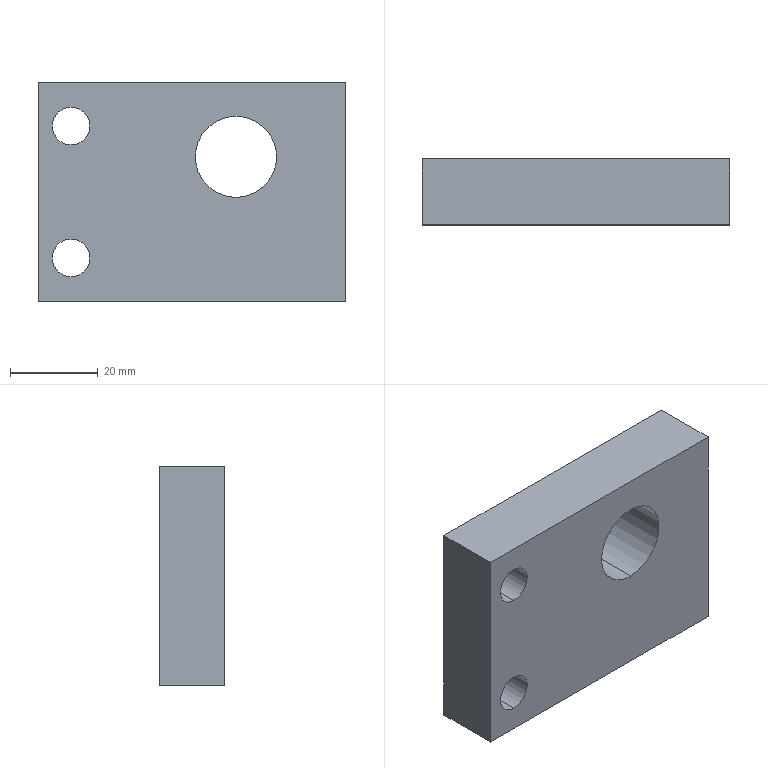Part | 1 solid | 12 faces | box 70 x 15 x 50 mm | volume 46725 mm3 | cylinder 6 | plane 6 | commonest cylinder face diameters 8.6 x4 18.5 x2
STEP:
#1=CARTESIAN_POINT('',(10.,0.,-9.75));
#2=VERTEX_POINT('',#1);
#3=CARTESIAN_POINT('',(10.,0.,8.75));
#4=VERTEX_POINT('',#3);
#5=CARTESIAN_POINT('',(10.,0.,-0.5));
#6=DIRECTION('',(0.,1.,0.));
#7=DIRECTION('',(0.,0.,1.));
#8=AXIS2_PLACEMENT_3D('',#5,#6,#7);
#9=CIRCLE('',#8,9.25);
#10=EDGE_CURVE('',#2,#4,#9,.T.);
#11=ORIENTED_EDGE('',*,*,#10,.F.);
#12=CARTESIAN_POINT('',(10.,15.,-9.75));
#13=VERTEX_POINT('',#12);
#14=CARTESIAN_POINT('',(10.,15.,-9.75));
#15=DIRECTION('',(0.,1.,0.));
#16=VECTOR('',#15,1000.);
#17=LINE('',#14,#16);
#18=EDGE_CURVE('',#2,#13,#17,.T.);
#19=ORIENTED_EDGE('',*,*,#18,.T.);
#20=CARTESIAN_POINT('',(10.,15.,8.75));
#21=VERTEX_POINT('',#20);
#22=CARTESIAN_POINT('',(10.,15.,-0.5));
#23=DIRECTION('',(0.,1.,0.));
#24=DIRECTION('',(0.,0.,1.));
#25=AXIS2_PLACEMENT_3D('',#22,#23,#24);
#26=CIRCLE('',#25,9.25);
#27=EDGE_CURVE('',#13,#21,#26,.T.);
#28=ORIENTED_EDGE('',*,*,#27,.T.);
#29=CARTESIAN_POINT('',(10.,15.,8.75));
#30=DIRECTION('',(0.,1.,0.));
#31=VECTOR('',#30,1000.);
#32=LINE('',#29,#31);
#33=EDGE_CURVE('',#4,#21,#32,.T.);
#34=ORIENTED_EDGE('',*,*,#33,.F.);
#35=EDGE_LOOP('',(#11,#19,#28,#34));
#36=FACE_OUTER_BOUND('',#35,.T.);
#37=CARTESIAN_POINT('',(10.,15.,-0.5));
#38=DIRECTION('',(0.,1.,0.));
#39=DIRECTION('',(0.,0.,1.));
#40=AXIS2_PLACEMENT_3D('',#37,#38,#39);
#41=CYLINDRICAL_SURFACE('',#40,9.25);
#42=ADVANCED_FACE('',(#36),#41,.F.);
#43=CARTESIAN_POINT('',(-27.5,0.,-27.8));
#44=VERTEX_POINT('',#43);
#45=CARTESIAN_POINT('',(-27.5,0.,-19.2));
#46=VERTEX_POINT('',#45);
#47=CARTESIAN_POINT('',(-27.5,0.,-23.5));
#48=DIRECTION('',(0.,1.,0.));
#49=DIRECTION('',(0.,0.,1.));
#50=AXIS2_PLACEMENT_3D('',#47,#48,#49);
#51=CIRCLE('',#50,4.3);
#52=EDGE_CURVE('',#44,#46,#51,.T.);
#53=ORIENTED_EDGE('',*,*,#52,.F.);
#54=CARTESIAN_POINT('',(-27.5,15.,-27.8));
#55=VERTEX_POINT('',#54);
#56=CARTESIAN_POINT('',(-27.5,0.,-27.8));
#57=DIRECTION('',(0.,1.,0.));
#58=VECTOR('',#57,1000.);
#59=LINE('',#56,#58);
#60=EDGE_CURVE('',#44,#55,#59,.T.);
#61=ORIENTED_EDGE('',*,*,#60,.T.);
#62=CARTESIAN_POINT('',(-27.5,15.,-19.2));
#63=VERTEX_POINT('',#62);
#64=CARTESIAN_POINT('',(-27.5,15.,-23.5));
#65=DIRECTION('',(0.,1.,0.));
#66=DIRECTION('',(0.,0.,1.));
#67=AXIS2_PLACEMENT_3D('',#64,#65,#66);
#68=CIRCLE('',#67,4.3);
#69=EDGE_CURVE('',#55,#63,#68,.T.);
#70=ORIENTED_EDGE('',*,*,#69,.T.);
#71=CARTESIAN_POINT('',(-27.5,0.,-19.2));
#72=DIRECTION('',(0.,1.,0.));
#73=VECTOR('',#72,1000.);
#74=LINE('',#71,#73);
#75=EDGE_CURVE('',#46,#63,#74,.T.);
#76=ORIENTED_EDGE('',*,*,#75,.F.);
#77=EDGE_LOOP('',(#53,#61,#70,#76));
#78=FACE_OUTER_BOUND('',#77,.T.);
#79=CARTESIAN_POINT('',(-27.5,0.,-23.5));
#80=DIRECTION('',(0.,1.,0.));
#81=DIRECTION('',(0.,0.,1.));
#82=AXIS2_PLACEMENT_3D('',#79,#80,#81);
#83=CYLINDRICAL_SURFACE('',#82,4.3);
#84=ADVANCED_FACE('',(#78),#83,.F.);
#85=CARTESIAN_POINT('',(-27.5,0.,2.2));
#86=VERTEX_POINT('',#85);
#87=CARTESIAN_POINT('',(-27.5,0.,10.8));
#88=VERTEX_POINT('',#87);
#89=CARTESIAN_POINT('',(-27.5,0.,6.5));
#90=DIRECTION('',(0.,1.,0.));
#91=DIRECTION('',(0.,0.,1.));
#92=AXIS2_PLACEMENT_3D('',#89,#90,#91);
#93=CIRCLE('',#92,4.3);
#94=EDGE_CURVE('',#86,#88,#93,.T.);
#95=ORIENTED_EDGE('',*,*,#94,.F.);
#96=CARTESIAN_POINT('',(-27.5,15.,2.2));
#97=VERTEX_POINT('',#96);
#98=CARTESIAN_POINT('',(-27.5,0.,2.2));
#99=DIRECTION('',(0.,1.,0.));
#100=VECTOR('',#99,1000.);
#101=LINE('',#98,#100);
#102=EDGE_CURVE('',#86,#97,#101,.T.);
#103=ORIENTED_EDGE('',*,*,#102,.T.);
#104=CARTESIAN_POINT('',(-27.5,15.,10.8));
#105=VERTEX_POINT('',#104);
#106=CARTESIAN_POINT('',(-27.5,15.,6.5));
#107=DIRECTION('',(0.,1.,0.));
#108=DIRECTION('',(0.,0.,1.));
#109=AXIS2_PLACEMENT_3D('',#106,#107,#108);
#110=CIRCLE('',#109,4.3);
#111=EDGE_CURVE('',#97,#105,#110,.T.);
#112=ORIENTED_EDGE('',*,*,#111,.T.);
#113=CARTESIAN_POINT('',(-27.5,0.,10.8));
#114=DIRECTION('',(0.,1.,0.));
#115=VECTOR('',#114,1000.);
#116=LINE('',#113,#115);
#117=EDGE_CURVE('',#88,#105,#116,.T.);
#118=ORIENTED_EDGE('',*,*,#117,.F.);
#119=EDGE_LOOP('',(#95,#103,#112,#118));
#120=FACE_OUTER_BOUND('',#119,.T.);
#121=CARTESIAN_POINT('',(-27.5,0.,6.5));
#122=DIRECTION('',(0.,1.,0.));
#123=DIRECTION('',(0.,0.,1.));
#124=AXIS2_PLACEMENT_3D('',#121,#122,#123);
#125=CYLINDRICAL_SURFACE('',#124,4.3);
#126=ADVANCED_FACE('',(#120),#125,.F.);
#127=CARTESIAN_POINT('',(35.,15.,16.5));
#128=VERTEX_POINT('',#127);
#129=CARTESIAN_POINT('',(35.,15.,-33.5));
#130=VERTEX_POINT('',#129);
#131=CARTESIAN_POINT('',(35.,15.,33.5));
#132=DIRECTION('',(0.,0.,-1.));
#133=VECTOR('',#132,1000.);
#134=LINE('',#131,#133);
#135=EDGE_CURVE('',#128,#130,#134,.T.);
#136=ORIENTED_EDGE('',*,*,#135,.F.);
#137=CARTESIAN_POINT('',(35.,0.,16.5));
#138=VERTEX_POINT('',#137);
#139=CARTESIAN_POINT('',(35.,0.,16.5));
#140=DIRECTION('',(0.,1.,0.));
#141=VECTOR('',#140,1000.);
#142=LINE('',#139,#141);
#143=EDGE_CURVE('',#138,#128,#142,.T.);
#144=ORIENTED_EDGE('',*,*,#143,.F.);
#145=CARTESIAN_POINT('',(35.,0.,-33.5));
#146=VERTEX_POINT('',#145);
#147=CARTESIAN_POINT('',(35.,0.,33.5));
#148=DIRECTION('',(0.,0.,-1.));
#149=VECTOR('',#148,1000.);
#150=LINE('',#147,#149);
#151=EDGE_CURVE('',#138,#146,#150,.T.);
#152=ORIENTED_EDGE('',*,*,#151,.T.);
#153=CARTESIAN_POINT('',(35.,15.,-33.5));
#154=DIRECTION('',(0.,-1.,0.));
#155=VECTOR('',#154,1000.);
#156=LINE('',#153,#155);
#157=EDGE_CURVE('',#130,#146,#156,.T.);
#158=ORIENTED_EDGE('',*,*,#157,.F.);
#159=EDGE_LOOP('',(#136,#144,#152,#158));
#160=FACE_OUTER_BOUND('',#159,.T.);
#161=CARTESIAN_POINT('',(35.,15.,33.5));
#162=DIRECTION('',(-1.,0.,0.));
#163=DIRECTION('',(0.,0.,1.));
#164=AXIS2_PLACEMENT_3D('',#161,#162,#163);
#165=PLANE('',#164);
#166=ADVANCED_FACE('',(#160),#165,.F.);
#167=CARTESIAN_POINT('',(-35.,0.,-33.5));
#168=VERTEX_POINT('',#167);
#169=CARTESIAN_POINT('',(-35.,0.,-33.5));
#170=DIRECTION('',(-1.,0.,0.));
#171=VECTOR('',#170,1000.);
#172=LINE('',#169,#171);
#173=EDGE_CURVE('',#146,#168,#172,.T.);
#174=ORIENTED_EDGE('',*,*,#173,.T.);
#175=CARTESIAN_POINT('',(-35.,15.,-33.5));
#176=VERTEX_POINT('',#175);
#177=CARTESIAN_POINT('',(-35.,15.,-33.5));
#178=DIRECTION('',(0.,-1.,0.));
#179=VECTOR('',#178,1000.);
#180=LINE('',#177,#179);
#181=EDGE_CURVE('',#176,#168,#180,.T.);
#182=ORIENTED_EDGE('',*,*,#181,.F.);
#183=CARTESIAN_POINT('',(-35.,15.,-33.5));
#184=DIRECTION('',(-1.,0.,0.));
#185=VECTOR('',#184,1000.);
#186=LINE('',#183,#185);
#187=EDGE_CURVE('',#130,#176,#186,.T.);
#188=ORIENTED_EDGE('',*,*,#187,.F.);
#189=ORIENTED_EDGE('',*,*,#157,.T.);
#190=EDGE_LOOP('',(#174,#182,#188,#189));
#191=FACE_OUTER_BOUND('',#190,.T.);
#192=CARTESIAN_POINT('',(-35.,15.,-33.5));
#193=DIRECTION('',(0.,0.,1.));
#194=DIRECTION('',(1.,0.,0.));
#195=AXIS2_PLACEMENT_3D('',#192,#193,#194);
#196=PLANE('',#195);
#197=ADVANCED_FACE('',(#191),#196,.F.);
#198=CARTESIAN_POINT('',(-35.,0.,16.5));
#199=VERTEX_POINT('',#198);
#200=CARTESIAN_POINT('',(-35.,0.,33.5));
#201=DIRECTION('',(0.,0.,1.));
#202=VECTOR('',#201,1000.);
#203=LINE('',#200,#202);
#204=EDGE_CURVE('',#168,#199,#203,.T.);
#205=ORIENTED_EDGE('',*,*,#204,.T.);
#206=CARTESIAN_POINT('',(-35.,15.,16.5));
#207=VERTEX_POINT('',#206);
#208=CARTESIAN_POINT('',(-35.,0.,16.5));
#209=DIRECTION('',(0.,1.,0.));
#210=VECTOR('',#209,1000.);
#211=LINE('',#208,#210);
#212=EDGE_CURVE('',#199,#207,#211,.T.);
#213=ORIENTED_EDGE('',*,*,#212,.T.);
#214=CARTESIAN_POINT('',(-35.,15.,33.5));
#215=DIRECTION('',(0.,0.,1.));
#216=VECTOR('',#215,1000.);
#217=LINE('',#214,#216);
#218=EDGE_CURVE('',#176,#207,#217,.T.);
#219=ORIENTED_EDGE('',*,*,#218,.F.);
#220=ORIENTED_EDGE('',*,*,#181,.T.);
#221=EDGE_LOOP('',(#205,#213,#219,#220));
#222=FACE_OUTER_BOUND('',#221,.T.);
#223=CARTESIAN_POINT('',(-35.,15.,33.5));
#224=DIRECTION('',(1.,0.,0.));
#225=DIRECTION('',(0.,0.,-1.));
#226=AXIS2_PLACEMENT_3D('',#223,#224,#225);
#227=PLANE('',#226);
#228=ADVANCED_FACE('',(#222),#227,.F.);
#229=CARTESIAN_POINT('',(10.,15.,-0.5));
#230=DIRECTION('',(0.,1.,0.));
#231=DIRECTION('',(0.,0.,1.));
#232=AXIS2_PLACEMENT_3D('',#229,#230,#231);
#233=CIRCLE('',#232,9.25);
#234=EDGE_CURVE('',#21,#13,#233,.T.);
#235=ORIENTED_EDGE('',*,*,#234,.F.);
#236=ORIENTED_EDGE('',*,*,#27,.F.);
#237=EDGE_LOOP('',(#235,#236));
#238=FACE_BOUND('',#237,.T.);
#239=CARTESIAN_POINT('',(-27.5,15.,-23.5));
#240=DIRECTION('',(0.,1.,0.));
#241=DIRECTION('',(0.,0.,1.));
#242=AXIS2_PLACEMENT_3D('',#239,#240,#241);
#243=CIRCLE('',#242,4.3);
#244=EDGE_CURVE('',#63,#55,#243,.T.);
#245=ORIENTED_EDGE('',*,*,#244,.F.);
#246=ORIENTED_EDGE('',*,*,#69,.F.);
#247=EDGE_LOOP('',(#245,#246));
#248=FACE_BOUND('',#247,.T.);
#249=CARTESIAN_POINT('',(-27.5,15.,6.5));
#250=DIRECTION('',(0.,1.,0.));
#251=DIRECTION('',(0.,0.,1.));
#252=AXIS2_PLACEMENT_3D('',#249,#250,#251);
#253=CIRCLE('',#252,4.3);
#254=EDGE_CURVE('',#105,#97,#253,.T.);
#255=ORIENTED_EDGE('',*,*,#254,.F.);
#256=ORIENTED_EDGE('',*,*,#111,.F.);
#257=EDGE_LOOP('',(#255,#256));
#258=FACE_BOUND('',#257,.T.);
#259=ORIENTED_EDGE('',*,*,#218,.T.);
#260=CARTESIAN_POINT('',(35.,15.,16.5));
#261=DIRECTION('',(-1.,0.,0.));
#262=VECTOR('',#261,1000.);
#263=LINE('',#260,#262);
#264=EDGE_CURVE('',#128,#207,#263,.T.);
#265=ORIENTED_EDGE('',*,*,#264,.F.);
#266=ORIENTED_EDGE('',*,*,#135,.T.);
#267=ORIENTED_EDGE('',*,*,#187,.T.);
#268=EDGE_LOOP('',(#259,#265,#266,#267));
#269=FACE_OUTER_BOUND('',#268,.T.);
#270=CARTESIAN_POINT('',(0.,15.,0.));
#271=DIRECTION('',(0.,-1.,0.));
#272=DIRECTION('',(0.,0.,-1.));
#273=AXIS2_PLACEMENT_3D('',#270,#271,#272);
#274=PLANE('',#273);
#275=ADVANCED_FACE('',(#238,#248,#258,#269),#274,.F.);
#276=CARTESIAN_POINT('',(35.,0.,16.5));
#277=DIRECTION('',(-1.,0.,0.));
#278=VECTOR('',#277,1000.);
#279=LINE('',#276,#278);
#280=EDGE_CURVE('',#138,#199,#279,.T.);
#281=ORIENTED_EDGE('',*,*,#280,.T.);
#282=ORIENTED_EDGE('',*,*,#204,.F.);
#283=ORIENTED_EDGE('',*,*,#173,.F.);
#284=ORIENTED_EDGE('',*,*,#151,.F.);
#285=EDGE_LOOP('',(#281,#282,#283,#284));
#286=FACE_OUTER_BOUND('',#285,.T.);
#287=CARTESIAN_POINT('',(10.,0.,-0.5));
#288=DIRECTION('',(0.,1.,0.));
#289=DIRECTION('',(0.,0.,1.));
#290=AXIS2_PLACEMENT_3D('',#287,#288,#289);
#291=CIRCLE('',#290,9.25);
#292=EDGE_CURVE('',#4,#2,#291,.T.);
#293=ORIENTED_EDGE('',*,*,#292,.T.);
#294=ORIENTED_EDGE('',*,*,#10,.T.);
#295=EDGE_LOOP('',(#293,#294));
#296=FACE_BOUND('',#295,.T.);
#297=CARTESIAN_POINT('',(-27.5,0.,-23.5));
#298=DIRECTION('',(0.,1.,0.));
#299=DIRECTION('',(0.,0.,1.));
#300=AXIS2_PLACEMENT_3D('',#297,#298,#299);
#301=CIRCLE('',#300,4.3);
#302=EDGE_CURVE('',#46,#44,#301,.T.);
#303=ORIENTED_EDGE('',*,*,#302,.T.);
#304=ORIENTED_EDGE('',*,*,#52,.T.);
#305=EDGE_LOOP('',(#303,#304));
#306=FACE_BOUND('',#305,.T.);
#307=CARTESIAN_POINT('',(-27.5,0.,6.5));
#308=DIRECTION('',(0.,1.,0.));
#309=DIRECTION('',(0.,0.,1.));
#310=AXIS2_PLACEMENT_3D('',#307,#308,#309);
#311=CIRCLE('',#310,4.3);
#312=EDGE_CURVE('',#88,#86,#311,.T.);
#313=ORIENTED_EDGE('',*,*,#312,.T.);
#314=ORIENTED_EDGE('',*,*,#94,.T.);
#315=EDGE_LOOP('',(#313,#314));
#316=FACE_BOUND('',#315,.T.);
#317=CARTESIAN_POINT('',(0.,0.,0.));
#318=DIRECTION('',(0.,-1.,0.));
#319=DIRECTION('',(0.,0.,-1.));
#320=AXIS2_PLACEMENT_3D('',#317,#318,#319);
#321=PLANE('',#320);
#322=ADVANCED_FACE('',(#286,#296,#306,#316),#321,.T.);
#323=ORIENTED_EDGE('',*,*,#102,.F.);
#324=ORIENTED_EDGE('',*,*,#312,.F.);
#325=ORIENTED_EDGE('',*,*,#117,.T.);
#326=ORIENTED_EDGE('',*,*,#254,.T.);
#327=EDGE_LOOP('',(#323,#324,#325,#326));
#328=FACE_OUTER_BOUND('',#327,.T.);
#329=CARTESIAN_POINT('',(-27.5,0.,6.5));
#330=DIRECTION('',(0.,1.,0.));
#331=DIRECTION('',(0.,0.,1.));
#332=AXIS2_PLACEMENT_3D('',#329,#330,#331);
#333=CYLINDRICAL_SURFACE('',#332,4.3);
#334=ADVANCED_FACE('',(#328),#333,.F.);
#335=ORIENTED_EDGE('',*,*,#60,.F.);
#336=ORIENTED_EDGE('',*,*,#302,.F.);
#337=ORIENTED_EDGE('',*,*,#75,.T.);
#338=ORIENTED_EDGE('',*,*,#244,.T.);
#339=EDGE_LOOP('',(#335,#336,#337,#338));
#340=FACE_OUTER_BOUND('',#339,.T.);
#341=CARTESIAN_POINT('',(-27.5,0.,-23.5));
#342=DIRECTION('',(0.,1.,0.));
#343=DIRECTION('',(0.,0.,1.));
#344=AXIS2_PLACEMENT_3D('',#341,#342,#343);
#345=CYLINDRICAL_SURFACE('',#344,4.3);
#346=ADVANCED_FACE('',(#340),#345,.F.);
#347=ORIENTED_EDGE('',*,*,#18,.F.);
#348=ORIENTED_EDGE('',*,*,#292,.F.);
#349=ORIENTED_EDGE('',*,*,#33,.T.);
#350=ORIENTED_EDGE('',*,*,#234,.T.);
#351=EDGE_LOOP('',(#347,#348,#349,#350));
#352=FACE_OUTER_BOUND('',#351,.T.);
#353=CARTESIAN_POINT('',(10.,15.,-0.5));
#354=DIRECTION('',(0.,1.,0.));
#355=DIRECTION('',(0.,0.,1.));
#356=AXIS2_PLACEMENT_3D('',#353,#354,#355);
#357=CYLINDRICAL_SURFACE('',#356,9.25);
#358=ADVANCED_FACE('',(#352),#357,.F.);
#359=ORIENTED_EDGE('',*,*,#264,.T.);
#360=ORIENTED_EDGE('',*,*,#212,.F.);
#361=ORIENTED_EDGE('',*,*,#280,.F.);
#362=ORIENTED_EDGE('',*,*,#143,.T.);
#363=EDGE_LOOP('',(#359,#360,#361,#362));
#364=FACE_OUTER_BOUND('',#363,.T.);
#365=CARTESIAN_POINT('',(35.,0.,16.5));
#366=DIRECTION('',(0.,0.,-1.));
#367=DIRECTION('',(-1.,0.,0.));
#368=AXIS2_PLACEMENT_3D('',#365,#366,#367);
#369=PLANE('',#368);
#370=ADVANCED_FACE('',(#364),#369,.F.);
#371=CLOSED_SHELL('',(#42,#84,#126,#166,#197,#228,#275,#322,#334,#346,#358,#370));
#372=MANIFOLD_SOLID_BREP('',#371);
#373=CARTESIAN_POINT('',(0.,0.,0.));
#374=DIRECTION('',(0.,0.,1.));
#375=DIRECTION('',(1.,0.,0.));
#376=AXIS2_PLACEMENT_3D('',#373,#374,#375);
#377=(LENGTH_UNIT()NAMED_UNIT(*)SI_UNIT(.MILLI.,.METRE.));
#378=UNCERTAINTY_MEASURE_WITH_UNIT(LENGTH_MEASURE(0.00001),#377,'','');
#379=(NAMED_UNIT(*)PLANE_ANGLE_UNIT()SI_UNIT($,.RADIAN.));
#380=(NAMED_UNIT(*)SI_UNIT($,.STERADIAN.)SOLID_ANGLE_UNIT());
#381=(GEOMETRIC_REPRESENTATION_CONTEXT(3)GLOBAL_UNCERTAINTY_ASSIGNED_CONTEXT((#378))GLOBAL_UNIT_ASSIGNED_CONTEXT((#377,#379,#380))REPRESENTATION_CONTEXT('',''));
#382=ADVANCED_BREP_SHAPE_REPRESENTATION('',(#372,#376),#381);